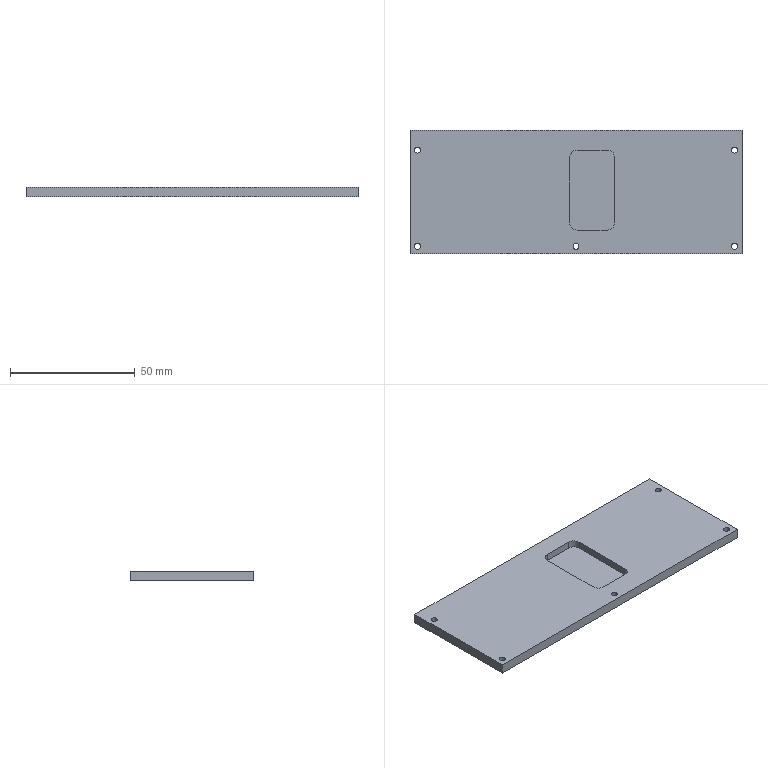NC program | NX | posted with a generic post | part box 133 x 49.5 x 4 mm
Whole program:
N10 G17 G21 G94 G90
(FLOOR_WALL , TOOL : D10JING)
N12 T09 M6
N14 G54
N16 G17 G0 G90 X-76.5 Y26.747 S9500 M3
N18 G43 Z30. H9
N20 Z3.
N22 G94 G1 Z0. F1250.
N24 X-73.5
N26 X73.5
N28 Y21.797
N30 X-73.5
N32 Y16.848
N34 X73.5
N36 Y11.898
N38 X-73.5
N40 Y6.948
N42 X73.5
N44 Y1.999
N46 X-73.5
N48 Y-2.951
N50 X73.5
N52 Y-7.901
N54 X-73.5
N56 Y-12.851
N58 X73.5
N60 Y-17.8
N62 X-73.5
N64 Y-17.997
N66 Y-22.75
N68 X73.5
N70 X76.5
N72 Z3.
N74 G0 Z30.
N76 M5
(DRILLING , TOOL : D6A45)
N78 T07 M6
N80 G54
N82 G17 G0 G90 X-63.5 Y16.75 S5000 M3
N84 G43 Z30. H7
N86 G94 G81 G98 Z-1.3 F250. R3.
N88 Y-21.75
N90 X0.
N92 X63.5
N94 Y16.75
N96 G80
N98 G0 X63.5 Y16.75 Z30.
N100 M5
(DRILLING_COPY , TOOL : 2.4ZT)
N102 T14 M6
N104 G54
N106 G17 G0 G90 X-63.5 Y16.75 S2000 M3
N108 G43 Z30. H14
N110 G94 G83 G98 Z-5.221 F150. Q2. R3.
N112 Y-21.75
N114 X0.
N116 X63.5
N118 Y16.75
N120 G80
N122 G0 X63.5 Y16.75 Z30.
N124 M5
(ZLEVEL_PROFILE , TOOL : D6)
N126 T06 M6
N128 G54
N130 G17 G0 G90 X-69.6 Y-4.626 S9500 M3
N132 G43 Z30. H6
N134 Z1.5
N136 G94 G1 Y25.182 Z-0.062 F1000.
N138 X-69.302 Y26.145 Z-0.115
N140 X-68.713 Y26.963 Z-0.168
N142 X-67.895 Y27.552 Z-0.221
N144 X-66.932 Y27.85 Z-0.273
N146 X-66.5 Z-0.296
N148 X66.5 F2500.
N150 G2 X69.6 Y24.75 R3.1
N152 G1 Y-24.75
N154 G2 X66.5 Y-27.85 R3.1
N156 G1 X-66.5
N158 G2 X-69.6 Y-24.75 R3.1
N160 G1 Y24.75
N162 G2 X-66.5 Y27.85 R3.1
N164 G1 X-49.533 Z-0.592
N166 X66.5
N168 G2 X69.6 Y24.75 R3.1
N170 G1 Y-24.75
N172 G2 X66.5 Y-27.85 R3.1
N174 G1 X-66.5
N176 G2 X-69.6 Y-24.75 R3.1
N178 G1 Y24.75
N180 G2 X-66.5 Y27.85 R3.1
N182 G1 X-49.533 Z-0.888
N184 X66.5
N186 G2 X69.6 Y24.75 R3.1
N188 G1 Y-24.75
N190 G2 X66.5 Y-27.85 R3.1
N192 G1 X-66.5
N194 G2 X-69.6 Y-24.75 R3.1
N196 G1 Y24.75
N198 G2 X-66.5 Y27.85 R3.1
N200 G1 X-49.533 Z-1.185
N202 X66.5
N204 G2 X69.6 Y24.75 R3.1
N206 G1 Y-24.75
N208 G2 X66.5 Y-27.85 R3.1
N210 G1 X-66.5
N212 G2 X-69.6 Y-24.75 R3.1
N214 G1 Y24.75
N216 G2 X-66.5 Y27.85 R3.1
N218 G1 X-49.533 Z-1.481
N220 X66.5
N222 G2 X69.6 Y24.75 R3.1
N224 G1 Y-24.75
N226 G2 X66.5 Y-27.85 R3.1
N228 G1 X-66.5
N230 G2 X-69.6 Y-24.75 R3.1
N232 G1 Y24.75
N234 G2 X-66.5 Y27.85 R3.1
N236 G1 X-49.533 Z-1.777
N238 X66.5
N240 G2 X69.6 Y24.75 R3.1
N242 G1 Y-24.75
N244 G2 X66.5 Y-27.85 R3.1
N246 G1 X-66.5
N248 G2 X-69.6 Y-24.75 R3.1
N250 G1 Y24.75
N252 G2 X-66.5 Y27.85 R3.1
N254 G1 X-49.533 Z-2.073
N256 X66.5
N258 G2 X69.6 Y24.75 R3.1
N260 G1 Y-24.75
N262 G2 X66.5 Y-27.85 R3.1
N264 G1 X-66.5
N266 G2 X-69.6 Y-24.75 R3.1
N268 G1 Y24.75
N270 G2 X-66.5 Y27.85 R3.1
N272 G1 X-49.533 Z-2.369
N274 X66.5
N276 G2 X69.6 Y24.75 R3.1
N278 G1 Y-24.75
N280 G2 X66.5 Y-27.85 R3.1
N282 G1 X-66.5
N284 G2 X-69.6 Y-24.75 R3.1
N286 G1 Y24.75
N288 G2 X-66.5 Y27.85 R3.1
N290 G1 X-49.533 Z-2.665
N292 X66.5
N294 G2 X69.6 Y24.75 R3.1
N296 G1 Y-24.75
N298 G2 X66.5 Y-27.85 R3.1
N300 G1 X-66.5
N302 G2 X-69.6 Y-24.75 R3.1
N304 G1 Y24.75
N306 G2 X-66.5 Y27.85 R3.1
N308 G1 X-49.533 Z-2.962
N310 X66.5
N312 G2 X69.6 Y24.75 R3.1
N314 G1 Y-24.75
N316 G2 X66.5 Y-27.85 R3.1
N318 G1 X-66.5
N320 G2 X-69.6 Y-24.75 R3.1
N322 G1 Y24.75
N324 G2 X-66.5 Y27.85 R3.1
N326 G1 X-49.533 Z-3.258
N328 X66.5
N330 G2 X69.6 Y24.75 R3.1
N332 G1 Y-24.75
N334 G2 X66.5 Y-27.85 R3.1
N336 G1 X-66.5
N338 G2 X-69.6 Y-24.75 R3.1
N340 G1 Y24.75
N342 G2 X-66.5 Y27.85 R3.1
N344 G1 X-49.533 Z-3.554
N346 X66.5
N348 G2 X69.6 Y24.75 R3.1
N350 G1 Y-24.75
N352 G2 X66.5 Y-27.85 R3.1
N354 G1 X-66.5
N356 G2 X-69.6 Y-24.75 R3.1
N358 G1 Y24.75
N360 G2 X-66.5 Y27.85 R3.1
N362 G1 X-49.533 Z-3.85
N364 X66.5
N366 G2 X69.6 Y24.75 R3.1
N368 G1 Y-24.75
N370 G2 X66.5 Y-27.85 R3.1
N372 G1 X-66.5
N374 G2 X-69.6 Y-24.75 R3.1
N376 G1 Y24.75
N378 G2 X-66.5 Y27.85 R3.1
N380 G1 X-49.533
N382 Z-2.35
N384 G0 Z30.
(FLOOR_WALL_1 , TOOL : D6)
N386 X6.7 Y5.735
N388 Z1.
N390 G1 Y7.95 Z0.884 F1000.
N392 X6.3 Z0.863
N394 Y-6.45 Z0.108
N396 X6.7 Z0.087
N398 Y0.75 Z-0.29
N400 Y7.95 F2500.
N402 X6.3
N404 Y-6.45
N406 X6.7
N408 Y0.75
N410 X9.4
N412 Y10.65
N414 X3.6
N416 Y-9.15
N418 X9.4
N420 Y0.75
N422 X12.4
N424 Y13.65
N426 X0.6
N428 Y-12.15
N430 X12.4
N432 Y0.75
N434 Z0.71
N436 G0 X6.7 Y5.735
N438 G1 Y7.95 Z0.594 F1000.
N440 X6.3 Z0.573
N442 Y-6.45 Z-0.182
N444 X6.7 Z-0.203
N446 Y0.75 Z-0.58
N448 Y7.95 F2500.
N450 X6.3
N452 Y-6.45
N454 X6.7
N456 Y0.75
N458 X9.4
N460 Y10.65
N462 X3.6
N464 Y-9.15
N466 X9.4
N468 Y0.75
N470 X12.4
N472 Y13.65
N474 X0.6
N476 Y-12.15
N478 X12.4
N480 Y0.75
N482 Z0.42
N484 G0 X6.7 Y5.735
N486 G1 Y7.95 Z0.304 F1000.
N488 X6.3 Z0.283
N490 Y-6.45 Z-0.472
N492 X6.7 Z-0.493
N494 Y0.75 Z-0.87
N496 Y7.95 F2500.
N498 X6.3
N500 Y-6.45
N502 X6.7
N504 Y0.75
N506 X9.4
N508 Y10.65
N510 X3.6
N512 Y-9.15
N514 X9.4
N516 Y0.75
N518 X12.4
N520 Y13.65
N522 X0.6
N524 Y-12.15
N526 X12.4
N528 Y0.75
N530 Z0.13
N532 G0 X6.7 Y5.735
N534 G1 Y7.95 Z0.014 F1000.
N536 X6.3 Z-0.007
N538 Y-6.45 Z-0.762
N540 X6.7 Z-0.783
N542 Y0.75 Z-1.16
N544 Y7.95 F2500.
N546 X6.3
N548 Y-6.45
N550 X6.7
N552 Y0.75
N554 X9.4
N556 Y10.65
N558 X3.6
N560 Y-9.15
N562 X9.4
N564 Y0.75
N566 X12.4
N568 Y13.65
N570 X0.6
N572 Y-12.15
N574 X12.4
N576 Y0.75
N578 Z-0.16
N580 G0 X6.7 Y5.735
N582 G1 Y7.95 Z-0.276 F1000.
N584 X6.3 Z-0.297
N586 Y-6.45 Z-1.052
N588 X6.7 Z-1.073
N590 Y0.75 Z-1.45
N592 Y7.95 F2500.
N594 X6.3
N596 Y-6.45
N598 X6.7
N600 Y0.75
N602 X9.4
N604 Y10.65
N606 X3.6
N608 Y-9.15
N610 X9.4
N612 Y0.75
N614 X12.4
N616 Y13.65
N618 X0.6
N620 Y-12.15
N622 X12.4
N624 Y0.75
N626 Z-0.45
N628 G0 X6.7 Y5.735
N630 G1 Y7.95 Z-0.566 F1000.
N632 X6.3 Z-0.587
N634 Y-6.45 Z-1.342
N636 X6.7 Z-1.363
N638 Y0.75 Z-1.74
N640 Y7.95 F2500.
N642 X6.3
N644 Y-6.45
N646 X6.7
N648 Y0.75
N650 X9.4
N652 Y10.65
N654 X3.6
N656 Y-9.15
N658 X9.4
N660 Y0.75
N662 X12.4
N664 Y13.65
N666 X0.6
N668 Y-12.15
N670 X12.4
N672 Y0.75
N674 Z-0.74
N676 G0 X6.7 Y5.735
N678 G1 Y7.95 Z-0.856 F1000.
N680 X6.3 Z-0.877
N682 Y-6.45 Z-1.632
N684 X6.7 Z-1.653
N686 Y0.75 Z-2.03
N688 Y7.95 F2500.
N690 X6.3
N692 Y-6.45
N694 X6.7
N696 Y0.75
N698 X9.4
N700 Y10.65
N702 X3.6
N704 Y-9.15
N706 X9.4
N708 Y0.75
N710 X12.4
N712 Y13.65
N714 X0.6
N716 Y-12.15
N718 X12.4
N720 Y0.75
N722 Z-1.03
N724 G0 X6.7 Y5.735
N726 G1 Y7.95 Z-1.146 F1000.
N728 X6.3 Z-1.167
N730 Y-6.45 Z-1.922
N732 X6.7 Z-1.943
N734 Y0.75 Z-2.32
N736 Y7.95 F2500.
N738 X6.3
N740 Y-6.45
N742 X6.7
N744 Y0.75
N746 X9.4
N748 Y10.65
N750 X3.6
N752 Y-9.15
N754 X9.4
N756 Y0.75
N758 X12.4
N760 Y13.65
N762 X0.6
N764 Y-12.15
N766 X12.4
N768 Y0.75
N770 Z-1.32
N772 G0 X6.7 Y5.735
N774 G1 Y7.95 Z-1.436 F1000.
N776 X6.3 Z-1.457
N778 Y-6.45 Z-2.212
N780 X6.7 Z-2.233
N782 Y0.75 Z-2.61
N784 Y7.95 F2500.
N786 X6.3
N788 Y-6.45
N790 X6.7
N792 Y0.75
N794 X9.4
N796 Y10.65
N798 X3.6
N800 Y-9.15
N802 X9.4
N804 Y0.75
N806 X12.4
N808 Y13.65
N810 X0.6
N812 Y-12.15
N814 X12.4
N816 Y0.75
N818 Z-1.61
N820 G0 X6.7 Y5.735
N822 G1 Y7.95 Z-1.726 F1000.
N824 X6.3 Z-1.747
N826 Y-6.45 Z-2.502
N828 X6.7 Z-2.523
N830 Y0.75 Z-2.9
N832 Y7.95 F2500.
N834 X6.3
N836 Y-6.45
N838 X6.7
N840 Y0.75
N842 X9.4
N844 Y10.65
N846 X3.6
N848 Y-9.15
N850 X9.4
N852 Y0.75
N854 X12.4
N856 Y13.65
N858 X0.6
N860 Y-12.15
N862 X12.4
N864 Y0.75
N866 Z-1.9
N868 G0 Z30.
(FLOOR_WALL_1_COPY , TOOL : D6)
N870 X1.1 Y1.27
N872 Z-2.
N874 G1 Z-3. F1000.
N876 G3 X0.8 Y0.75 R0.6
N878 G1 Y13.45 F1200.
N880 X12.2
N882 Y-11.95
N884 X0.8
N886 Y0.75
N888 X3.8
N890 Y10.45
N892 X9.2
N894 Y-8.95
N896 X3.8
N898 Y0.75
N900 X6.5
N902 Y7.75
N904 Y-6.25
N906 Y0.75
N908 X0.8 Y1.27
N910 G3 X0.5 Y0.75 R0.6 F1000.
N912 G1 Y-12.25 F1200.
N914 X12.5
N916 Y13.75
N918 X0.5
N920 Y0.75
N922 G3 X0.8 Y0.23 R0.6
N924 G1 X2.5 Y-0.751
N926 Z-2.
N928 G0 Z30.
N930 M5
(ZLEVEL_PROFILE_1_COPY , TOOL : D6A45)
N932 T07 M6
N934 G54
N936 G17 G0 G90 X-63.741 Y16.75 S9500 M3
N938 G43 Z30. H7
N940 Z2.
N942 G94 G1 Z-1. F1250.
N944 X-63.733 Y16.687
N946 G3 X-63.741 Y16.75 R-0.241
N948 G1 X-63.76 Y16.665
N950 X-63.701 Y16.6
N952 Z1.
N954 G0 Z30.
N956 X-0.306 Y13.991
N958 Z1.
N960 G1 Z-1.
N962 X-1.241 Y14.27
N964 G3 X-1.541 Y13.75 R0.6
N966 G1 Y-12.25
N968 G3 X0.5 Y-14.291 R2.041
N970 G1 X12.5
N972 G3 X14.541 Y-12.25 R2.041
N974 G1 Y13.75
N976 G3 X12.5 Y15.791 R2.041
N978 G1 X0.5
N980 G3 X-1.541 Y13.75 R2.041
N982 X-1.241 Y13.23 R0.6
N984 G1 X-0.341 Y12.711
N986 Z1.
N988 G0 Z30.
N990 X63.741 Y-21.75
N992 Z2.
N994 G1 Z-1.
N996 Y-21.749
N998 G3 X63.499 Y-21.509 R0.241
N1000 X63.741 Y-21.75 R-0.241
N1002 G1 X63.76 Y-21.665
N1004 X63.701 Y-21.6
N1006 Z1.
N1008 G0 Z30.
N1010 X0. Y-21.991
N1012 Z2.
N1014 G1 Z-1.
N1016 G3 X0.241 Y-21.75 R0.241
N1018 X0. Y-21.991 R-0.241
N1020 G1 X0.085 Y-22.01
N1022 X0.15 Y-21.951
N1024 Z1.
N1026 G0 Z30.
N1028 X-63.741 Y-21.75
N1030 Z2.
N1032 G1 Z-1.
N1034 G3 X-63.5 Y-21.991 R0.241
N1036 X-63.741 Y-21.75 R-0.241
N1038 G1 X-63.76 Y-21.835
N1040 X-63.701 Y-21.9
N1042 Z1.
N1044 G0 Z30.
N1046 X63.741 Y16.75
N1048 Z2.
N1050 G1 Z-1.
N1052 Y16.764
N1054 G3 X63.741 Y16.75 R-0.241
N1056 G1 X63.76 Y16.835
N1058 X63.701 Y16.9
N1060 Z1.
N1062 G0 Z30.
N1064 X-67.419 Y26.696
N1066 Z1.
N1068 G1 Z-1.
N1070 X-67.022 Y26.009
N1072 G3 X-66.503 Y25.709 R0.6
N1074 G1 X66.503
N1076 G2 X67.459 Y24.753 R0.98
N1078 G1 Y-24.753
N1080 G2 X66.503 Y-25.709 R0.98
N1082 G1 X-66.503
N1084 G2 X-67.459 Y-24.753 R0.98
N1086 G1 Y24.753
N1088 G2 X-66.503 Y25.709 R0.98
N1090 G3 X-65.99 Y26.021 R0.6
N1092 G1 X-65.506 Y26.909
N1094 Z1.
N1096 G0 Z30.
N1098 M5
(刀补 , TOOL : D6)
N1100 T06 M6
N1102 G54
N1104 G17 G0 G90 X67.507 Y-28.93 S9500 M3
N1106 G43 Z30. H6
N1108 Z-2.35
N1110 G94 G1 Z-3.85 F1000.
N1112 G41 X67.473 Y-28.836 D6
N1114 X67.02 Y-28.05
N1116 G3 X66.5 Y-27.75 R0.6
N1118 G1 X-66.5 F1200.
N1120 G2 X-69.5 Y-24.75 R3.
N1122 G1 Y24.75
N1124 G2 X-66.5 Y27.75 R3.
N1126 G1 X66.5
N1128 G2 X69.5 Y24.75 R3.
N1130 G1 Y-24.75
N1132 G2 X66.5 Y-27.75 R3.
N1134 G3 X65.98 Y-28.05 R0.6
N1136 G1 X65.461 Y-28.95
N1138 G40
N1140 X65.427 Y-29.044
N1142 Z-2.35
N1144 G0 Z30.
N1146 M5
N1148 M2